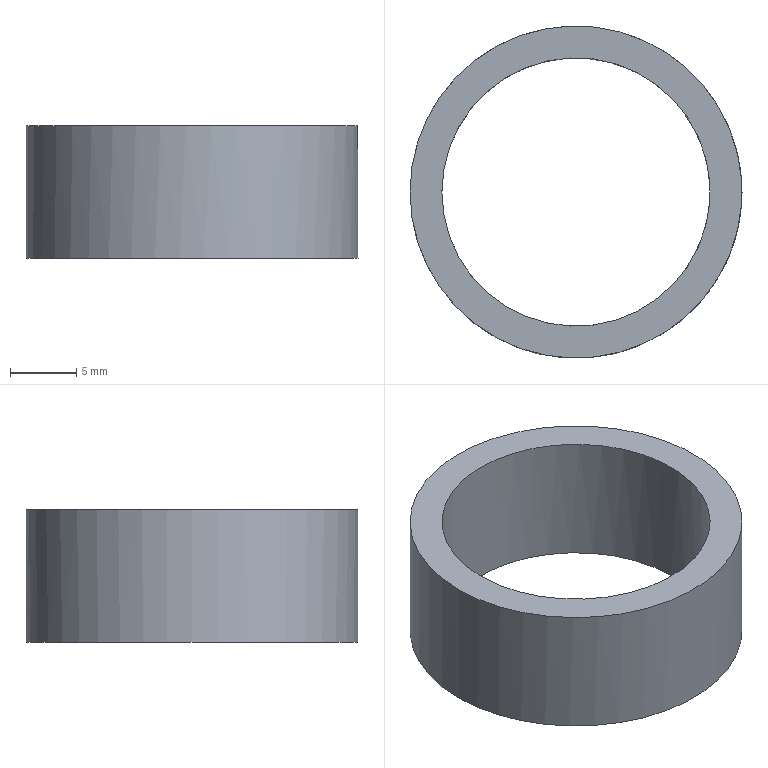Part | NX | features DATUM_CSYS 1, EXTRACT_DATUM_PLANE 1, EXTRUDE 1, SKETCH 1 | 1 solid | 4 faces | box 25 x 25 x 10 mm | volume 1704 mm3 | cylinder 2 | plane 2 | commonest cylinder face diameters 20.2 x1 25 x1
STEP:
#1=CARTESIAN_POINT('',(12.5,0.,0.));
#2=VERTEX_POINT('',#1);
#3=CARTESIAN_POINT('',(0.,0.,0.));
#4=DIRECTION('',(0.,0.,-1.));
#5=DIRECTION('',(1.,0.,0.));
#6=AXIS2_PLACEMENT_3D('',#3,#4,#5);
#7=CIRCLE('',#6,12.5);
#8=EDGE_CURVE('',#2,#2,#7,.T.);
#9=ORIENTED_EDGE('',*,*,#8,.F.);
#10=EDGE_LOOP('',(#9));
#11=FACE_BOUND('',#10,.T.);
#12=CARTESIAN_POINT('',(-12.5,0.,10.));
#13=VERTEX_POINT('',#12);
#14=CARTESIAN_POINT('',(0.,0.,10.));
#15=DIRECTION('',(0.,0.,-1.));
#16=DIRECTION('',(-1.,0.,0.));
#17=AXIS2_PLACEMENT_3D('',#14,#15,#16);
#18=CIRCLE('',#17,12.5);
#19=EDGE_CURVE('',#13,#13,#18,.T.);
#20=ORIENTED_EDGE('',*,*,#19,.T.);
#21=EDGE_LOOP('',(#20));
#22=FACE_BOUND('',#21,.T.);
#23=CARTESIAN_POINT('',(0.,0.,10.));
#24=DIRECTION('',(0.,0.,-1.));
#25=DIRECTION('',(-1.,0.,0.));
#26=AXIS2_PLACEMENT_3D('',#23,#24,#25);
#27=CYLINDRICAL_SURFACE('',#26,12.5);
#28=ADVANCED_FACE('',(#11,#22),#27,.T.);
#29=CARTESIAN_POINT('',(10.1,0.,0.));
#30=VERTEX_POINT('',#29);
#31=CARTESIAN_POINT('',(0.,0.,0.));
#32=DIRECTION('',(0.,0.,1.));
#33=DIRECTION('',(1.,0.,0.));
#34=AXIS2_PLACEMENT_3D('',#31,#32,#33);
#35=CIRCLE('',#34,10.1);
#36=EDGE_CURVE('',#30,#30,#35,.T.);
#37=ORIENTED_EDGE('',*,*,#36,.F.);
#38=EDGE_LOOP('',(#37));
#39=FACE_BOUND('',#38,.T.);
#40=CARTESIAN_POINT('',(-10.1,0.,10.));
#41=VERTEX_POINT('',#40);
#42=CARTESIAN_POINT('',(0.,0.,10.));
#43=DIRECTION('',(0.,0.,1.));
#44=DIRECTION('',(-1.,0.,0.));
#45=AXIS2_PLACEMENT_3D('',#42,#43,#44);
#46=CIRCLE('',#45,10.1);
#47=EDGE_CURVE('',#41,#41,#46,.T.);
#48=ORIENTED_EDGE('',*,*,#47,.T.);
#49=EDGE_LOOP('',(#48));
#50=FACE_BOUND('',#49,.T.);
#51=CARTESIAN_POINT('',(0.,0.,10.));
#52=DIRECTION('',(0.,0.,-1.));
#53=DIRECTION('',(-1.,0.,0.));
#54=AXIS2_PLACEMENT_3D('',#51,#52,#53);
#55=CYLINDRICAL_SURFACE('',#54,10.1);
#56=ADVANCED_FACE('',(#39,#50),#55,.F.);
#57=ORIENTED_EDGE('',*,*,#19,.F.);
#58=EDGE_LOOP('',(#57));
#59=FACE_BOUND('',#58,.T.);
#60=ORIENTED_EDGE('',*,*,#47,.F.);
#61=EDGE_LOOP('',(#60));
#62=FACE_BOUND('',#61,.T.);
#63=CARTESIAN_POINT('',(0.,0.,10.));
#64=DIRECTION('',(0.,0.,-1.));
#65=DIRECTION('',(-1.,0.,0.));
#66=AXIS2_PLACEMENT_3D('',#63,#64,#65);
#67=PLANE('',#66);
#68=ADVANCED_FACE('',(#59,#62),#67,.F.);
#69=ORIENTED_EDGE('',*,*,#8,.T.);
#70=EDGE_LOOP('',(#69));
#71=FACE_BOUND('',#70,.T.);
#72=ORIENTED_EDGE('',*,*,#36,.T.);
#73=EDGE_LOOP('',(#72));
#74=FACE_BOUND('',#73,.T.);
#75=CARTESIAN_POINT('',(0.,0.,0.));
#76=DIRECTION('',(0.,0.,-1.));
#77=DIRECTION('',(-1.,0.,0.));
#78=AXIS2_PLACEMENT_3D('',#75,#76,#77);
#79=PLANE('',#78);
#80=ADVANCED_FACE('',(#71,#74),#79,.T.);
#81=CLOSED_SHELL('',(#28,#56,#68,#80));
#82=MANIFOLD_SOLID_BREP('',#81);
#83=(LENGTH_UNIT()NAMED_UNIT(*)SI_UNIT(.MILLI.,.METRE.));
#84=UNCERTAINTY_MEASURE_WITH_UNIT(LENGTH_MEASURE(0.00001),#83,'','');
#85=(NAMED_UNIT(*)PLANE_ANGLE_UNIT()SI_UNIT($,.RADIAN.));
#86=(NAMED_UNIT(*)SI_UNIT($,.STERADIAN.)SOLID_ANGLE_UNIT());
#87=(GEOMETRIC_REPRESENTATION_CONTEXT(3)GLOBAL_UNCERTAINTY_ASSIGNED_CONTEXT((#84))GLOBAL_UNIT_ASSIGNED_CONTEXT((#83,#85,#86))REPRESENTATION_CONTEXT('',''));
#88=ADVANCED_BREP_SHAPE_REPRESENTATION('',(#82),#87);